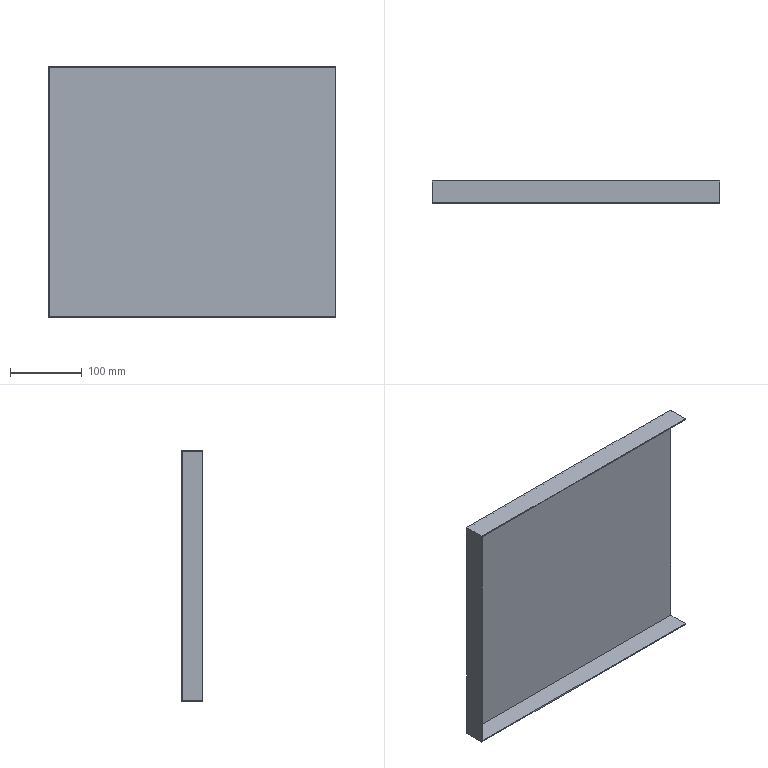Part | STEP file | B-BAN1_1-2 | 1 solid | 10 faces | box 400 x 30 x 350 mm | volume 259034 mm3 | plane 10
STEP:
#1=CARTESIAN_POINT('',(200.,30.,-175.));
#2=VERTEX_POINT('',#1);
#3=CARTESIAN_POINT('',(-200.,30.,-175.));
#4=VERTEX_POINT('',#3);
#5=CARTESIAN_POINT('',(0.,30.,-175.));
#6=DIRECTION('',(-1.,0.,0.));
#7=VECTOR('',#6,1000.);
#8=LINE('',#5,#7);
#9=EDGE_CURVE('',#2,#4,#8,.T.);
#10=ORIENTED_EDGE('',*,*,#9,.T.);
#11=CARTESIAN_POINT('',(-200.,30.,175.));
#12=VERTEX_POINT('',#11);
#13=CARTESIAN_POINT('',(-200.,30.,0.));
#14=DIRECTION('',(0.,0.,1.));
#15=VECTOR('',#14,1000.);
#16=LINE('',#13,#15);
#17=EDGE_CURVE('',#4,#12,#16,.T.);
#18=ORIENTED_EDGE('',*,*,#17,.T.);
#19=CARTESIAN_POINT('',(200.,30.,175.));
#20=VERTEX_POINT('',#19);
#21=CARTESIAN_POINT('',(0.,30.,175.));
#22=DIRECTION('',(1.,0.,0.));
#23=VECTOR('',#22,1000.);
#24=LINE('',#21,#23);
#25=EDGE_CURVE('',#12,#20,#24,.T.);
#26=ORIENTED_EDGE('',*,*,#25,.T.);
#27=CARTESIAN_POINT('',(200.,30.,0.));
#28=DIRECTION('',(0.,0.,-1.));
#29=VECTOR('',#28,1000.);
#30=LINE('',#27,#29);
#31=EDGE_CURVE('',#20,#2,#30,.T.);
#32=ORIENTED_EDGE('',*,*,#31,.T.);
#33=EDGE_LOOP('',(#10,#18,#26,#32));
#34=FACE_OUTER_BOUND('',#33,.T.);
#35=CARTESIAN_POINT('',(0.,30.,0.));
#36=DIRECTION('',(0.,1.,0.));
#37=DIRECTION('',(0.,0.,1.));
#38=AXIS2_PLACEMENT_3D('',#35,#36,#37);
#39=PLANE('',#38);
#40=ADVANCED_FACE('',(#34),#39,.T.);
#41=CARTESIAN_POINT('',(-200.,0.,-175.));
#42=VERTEX_POINT('',#41);
#43=CARTESIAN_POINT('',(-200.,0.,-175.));
#44=DIRECTION('',(0.,-1.,0.));
#45=VECTOR('',#44,1000.);
#46=LINE('',#43,#45);
#47=EDGE_CURVE('',#4,#42,#46,.T.);
#48=ORIENTED_EDGE('',*,*,#47,.T.);
#49=CARTESIAN_POINT('',(-200.,0.,175.));
#50=VERTEX_POINT('',#49);
#51=CARTESIAN_POINT('',(-200.,0.,-175.));
#52=DIRECTION('',(0.,0.,1.));
#53=VECTOR('',#52,1000.);
#54=LINE('',#51,#53);
#55=EDGE_CURVE('',#42,#50,#54,.T.);
#56=ORIENTED_EDGE('',*,*,#55,.T.);
#57=CARTESIAN_POINT('',(-200.,0.,175.));
#58=DIRECTION('',(0.,1.,0.));
#59=VECTOR('',#58,1000.);
#60=LINE('',#57,#59);
#61=EDGE_CURVE('',#50,#12,#60,.T.);
#62=ORIENTED_EDGE('',*,*,#61,.T.);
#63=ORIENTED_EDGE('',*,*,#17,.F.);
#64=EDGE_LOOP('',(#48,#56,#62,#63));
#65=FACE_OUTER_BOUND('',#64,.T.);
#66=CARTESIAN_POINT('',(-200.,0.,-175.));
#67=DIRECTION('',(-1.,0.,0.));
#68=DIRECTION('',(0.,0.,1.));
#69=AXIS2_PLACEMENT_3D('',#66,#67,#68);
#70=PLANE('',#69);
#71=ADVANCED_FACE('',(#65),#70,.T.);
#72=CARTESIAN_POINT('',(200.,0.,-175.));
#73=VERTEX_POINT('',#72);
#74=CARTESIAN_POINT('',(200.,0.,-175.));
#75=DIRECTION('',(0.,-1.,0.));
#76=VECTOR('',#75,1000.);
#77=LINE('',#74,#76);
#78=EDGE_CURVE('',#2,#73,#77,.T.);
#79=ORIENTED_EDGE('',*,*,#78,.T.);
#80=CARTESIAN_POINT('',(200.,0.,-175.));
#81=DIRECTION('',(-1.,0.,0.));
#82=VECTOR('',#81,1000.);
#83=LINE('',#80,#82);
#84=EDGE_CURVE('',#73,#42,#83,.T.);
#85=ORIENTED_EDGE('',*,*,#84,.T.);
#86=ORIENTED_EDGE('',*,*,#47,.F.);
#87=ORIENTED_EDGE('',*,*,#9,.F.);
#88=EDGE_LOOP('',(#79,#85,#86,#87));
#89=FACE_OUTER_BOUND('',#88,.T.);
#90=CARTESIAN_POINT('',(200.,0.,-175.));
#91=DIRECTION('',(0.,0.,-1.));
#92=DIRECTION('',(-1.,0.,0.));
#93=AXIS2_PLACEMENT_3D('',#90,#91,#92);
#94=PLANE('',#93);
#95=ADVANCED_FACE('',(#89),#94,.T.);
#96=CARTESIAN_POINT('',(200.,0.,173.5));
#97=VERTEX_POINT('',#96);
#98=CARTESIAN_POINT('',(200.,28.5,173.5));
#99=VERTEX_POINT('',#98);
#100=CARTESIAN_POINT('',(200.,0.,173.5));
#101=DIRECTION('',(0.,1.,0.));
#102=VECTOR('',#101,1000.);
#103=LINE('',#100,#102);
#104=EDGE_CURVE('',#97,#99,#103,.T.);
#105=ORIENTED_EDGE('',*,*,#104,.T.);
#106=CARTESIAN_POINT('',(200.,28.5,-173.5));
#107=VERTEX_POINT('',#106);
#108=CARTESIAN_POINT('',(200.,28.5,175.));
#109=DIRECTION('',(0.,0.,-1.));
#110=VECTOR('',#109,1000.);
#111=LINE('',#108,#110);
#112=EDGE_CURVE('',#99,#107,#111,.T.);
#113=ORIENTED_EDGE('',*,*,#112,.T.);
#114=CARTESIAN_POINT('',(200.,0.,-173.5));
#115=VERTEX_POINT('',#114);
#116=CARTESIAN_POINT('',(200.,0.,-173.5));
#117=DIRECTION('',(0.,-1.,0.));
#118=VECTOR('',#117,1000.);
#119=LINE('',#116,#118);
#120=EDGE_CURVE('',#107,#115,#119,.T.);
#121=ORIENTED_EDGE('',*,*,#120,.T.);
#122=CARTESIAN_POINT('',(200.,0.,175.));
#123=DIRECTION('',(0.,0.,-1.));
#124=VECTOR('',#123,1000.);
#125=LINE('',#122,#124);
#126=EDGE_CURVE('',#115,#73,#125,.T.);
#127=ORIENTED_EDGE('',*,*,#126,.T.);
#128=ORIENTED_EDGE('',*,*,#78,.F.);
#129=ORIENTED_EDGE('',*,*,#31,.F.);
#130=CARTESIAN_POINT('',(200.,0.,175.));
#131=VERTEX_POINT('',#130);
#132=CARTESIAN_POINT('',(200.,0.,175.));
#133=DIRECTION('',(0.,-1.,0.));
#134=VECTOR('',#133,1000.);
#135=LINE('',#132,#134);
#136=EDGE_CURVE('',#20,#131,#135,.T.);
#137=ORIENTED_EDGE('',*,*,#136,.T.);
#138=CARTESIAN_POINT('',(200.,0.,175.));
#139=DIRECTION('',(0.,0.,-1.));
#140=VECTOR('',#139,1000.);
#141=LINE('',#138,#140);
#142=EDGE_CURVE('',#131,#97,#141,.T.);
#143=ORIENTED_EDGE('',*,*,#142,.T.);
#144=EDGE_LOOP('',(#105,#113,#121,#127,#128,#129,#137,#143));
#145=FACE_OUTER_BOUND('',#144,.T.);
#146=CARTESIAN_POINT('',(200.,0.,175.));
#147=DIRECTION('',(1.,0.,0.));
#148=DIRECTION('',(0.,0.,-1.));
#149=AXIS2_PLACEMENT_3D('',#146,#147,#148);
#150=PLANE('',#149);
#151=ADVANCED_FACE('',(#145),#150,.T.);
#152=ORIENTED_EDGE('',*,*,#61,.F.);
#153=CARTESIAN_POINT('',(-200.,0.,175.));
#154=DIRECTION('',(1.,0.,0.));
#155=VECTOR('',#154,1000.);
#156=LINE('',#153,#155);
#157=EDGE_CURVE('',#50,#131,#156,.T.);
#158=ORIENTED_EDGE('',*,*,#157,.T.);
#159=ORIENTED_EDGE('',*,*,#136,.F.);
#160=ORIENTED_EDGE('',*,*,#25,.F.);
#161=EDGE_LOOP('',(#152,#158,#159,#160));
#162=FACE_OUTER_BOUND('',#161,.T.);
#163=CARTESIAN_POINT('',(-200.,0.,175.));
#164=DIRECTION('',(0.,0.,1.));
#165=DIRECTION('',(1.,0.,0.));
#166=AXIS2_PLACEMENT_3D('',#163,#164,#165);
#167=PLANE('',#166);
#168=ADVANCED_FACE('',(#162),#167,.T.);
#169=ORIENTED_EDGE('',*,*,#142,.F.);
#170=ORIENTED_EDGE('',*,*,#157,.F.);
#171=ORIENTED_EDGE('',*,*,#55,.F.);
#172=ORIENTED_EDGE('',*,*,#84,.F.);
#173=ORIENTED_EDGE('',*,*,#126,.F.);
#174=CARTESIAN_POINT('',(-198.5,0.,-173.5));
#175=VERTEX_POINT('',#174);
#176=CARTESIAN_POINT('',(0.,0.,-173.5));
#177=DIRECTION('',(1.,0.,0.));
#178=VECTOR('',#177,1000.);
#179=LINE('',#176,#178);
#180=EDGE_CURVE('',#175,#115,#179,.T.);
#181=ORIENTED_EDGE('',*,*,#180,.F.);
#182=CARTESIAN_POINT('',(-198.5,0.,173.5));
#183=VERTEX_POINT('',#182);
#184=CARTESIAN_POINT('',(-198.5,0.,0.));
#185=DIRECTION('',(0.,0.,-1.));
#186=VECTOR('',#185,1000.);
#187=LINE('',#184,#186);
#188=EDGE_CURVE('',#183,#175,#187,.T.);
#189=ORIENTED_EDGE('',*,*,#188,.F.);
#190=CARTESIAN_POINT('',(0.,0.,173.5));
#191=DIRECTION('',(-1.,0.,0.));
#192=VECTOR('',#191,1000.);
#193=LINE('',#190,#192);
#194=EDGE_CURVE('',#97,#183,#193,.T.);
#195=ORIENTED_EDGE('',*,*,#194,.F.);
#196=EDGE_LOOP('',(#169,#170,#171,#172,#173,#181,#189,#195));
#197=FACE_OUTER_BOUND('',#196,.T.);
#198=CARTESIAN_POINT('',(0.,0.,0.));
#199=DIRECTION('',(0.,1.,0.));
#200=DIRECTION('',(0.,0.,1.));
#201=AXIS2_PLACEMENT_3D('',#198,#199,#200);
#202=PLANE('',#201);
#203=ADVANCED_FACE('',(#197),#202,.F.);
#204=CARTESIAN_POINT('',(-198.5,28.5,-173.5));
#205=VERTEX_POINT('',#204);
#206=CARTESIAN_POINT('',(-198.5,28.5,173.5));
#207=VERTEX_POINT('',#206);
#208=CARTESIAN_POINT('',(-198.5,28.5,0.));
#209=DIRECTION('',(0.,0.,1.));
#210=VECTOR('',#209,1000.);
#211=LINE('',#208,#210);
#212=EDGE_CURVE('',#205,#207,#211,.T.);
#213=ORIENTED_EDGE('',*,*,#212,.F.);
#214=CARTESIAN_POINT('',(0.,28.5,-173.5));
#215=DIRECTION('',(-1.,0.,0.));
#216=VECTOR('',#215,1000.);
#217=LINE('',#214,#216);
#218=EDGE_CURVE('',#107,#205,#217,.T.);
#219=ORIENTED_EDGE('',*,*,#218,.F.);
#220=ORIENTED_EDGE('',*,*,#112,.F.);
#221=CARTESIAN_POINT('',(0.,28.5,173.5));
#222=DIRECTION('',(1.,0.,0.));
#223=VECTOR('',#222,1000.);
#224=LINE('',#221,#223);
#225=EDGE_CURVE('',#207,#99,#224,.T.);
#226=ORIENTED_EDGE('',*,*,#225,.F.);
#227=EDGE_LOOP('',(#213,#219,#220,#226));
#228=FACE_OUTER_BOUND('',#227,.T.);
#229=CARTESIAN_POINT('',(0.,28.5,0.));
#230=DIRECTION('',(0.,1.,0.));
#231=DIRECTION('',(0.,0.,1.));
#232=AXIS2_PLACEMENT_3D('',#229,#230,#231);
#233=PLANE('',#232);
#234=ADVANCED_FACE('',(#228),#233,.F.);
#235=ORIENTED_EDGE('',*,*,#225,.T.);
#236=ORIENTED_EDGE('',*,*,#104,.F.);
#237=ORIENTED_EDGE('',*,*,#194,.T.);
#238=CARTESIAN_POINT('',(-198.5,0.,173.5));
#239=DIRECTION('',(0.,-1.,0.));
#240=VECTOR('',#239,1000.);
#241=LINE('',#238,#240);
#242=EDGE_CURVE('',#207,#183,#241,.T.);
#243=ORIENTED_EDGE('',*,*,#242,.F.);
#244=EDGE_LOOP('',(#235,#236,#237,#243));
#245=FACE_OUTER_BOUND('',#244,.T.);
#246=CARTESIAN_POINT('',(-200.,0.,173.5));
#247=DIRECTION('',(0.,0.,1.));
#248=DIRECTION('',(1.,0.,0.));
#249=AXIS2_PLACEMENT_3D('',#246,#247,#248);
#250=PLANE('',#249);
#251=ADVANCED_FACE('',(#245),#250,.F.);
#252=ORIENTED_EDGE('',*,*,#218,.T.);
#253=CARTESIAN_POINT('',(-198.5,0.,-173.5));
#254=DIRECTION('',(0.,1.,0.));
#255=VECTOR('',#254,1000.);
#256=LINE('',#253,#255);
#257=EDGE_CURVE('',#175,#205,#256,.T.);
#258=ORIENTED_EDGE('',*,*,#257,.F.);
#259=ORIENTED_EDGE('',*,*,#180,.T.);
#260=ORIENTED_EDGE('',*,*,#120,.F.);
#261=EDGE_LOOP('',(#252,#258,#259,#260));
#262=FACE_OUTER_BOUND('',#261,.T.);
#263=CARTESIAN_POINT('',(200.,0.,-173.5));
#264=DIRECTION('',(0.,0.,-1.));
#265=DIRECTION('',(-1.,0.,0.));
#266=AXIS2_PLACEMENT_3D('',#263,#264,#265);
#267=PLANE('',#266);
#268=ADVANCED_FACE('',(#262),#267,.F.);
#269=ORIENTED_EDGE('',*,*,#212,.T.);
#270=ORIENTED_EDGE('',*,*,#242,.T.);
#271=ORIENTED_EDGE('',*,*,#188,.T.);
#272=ORIENTED_EDGE('',*,*,#257,.T.);
#273=EDGE_LOOP('',(#269,#270,#271,#272));
#274=FACE_OUTER_BOUND('',#273,.T.);
#275=CARTESIAN_POINT('',(-198.5,0.,-175.));
#276=DIRECTION('',(-1.,0.,0.));
#277=DIRECTION('',(0.,0.,1.));
#278=AXIS2_PLACEMENT_3D('',#275,#276,#277);
#279=PLANE('',#278);
#280=ADVANCED_FACE('',(#274),#279,.F.);
#281=CLOSED_SHELL('',(#40,#71,#95,#151,#168,#203,#234,#251,#268,#280));
#282=MANIFOLD_SOLID_BREP('',#281);
#283=CARTESIAN_POINT('',(0.,0.,0.));
#284=DIRECTION('',(0.,0.,1.));
#285=DIRECTION('',(1.,0.,0.));
#286=AXIS2_PLACEMENT_3D('',#283,#284,#285);
#287=(LENGTH_UNIT()NAMED_UNIT(*)SI_UNIT(.MILLI.,.METRE.));
#288=UNCERTAINTY_MEASURE_WITH_UNIT(LENGTH_MEASURE(0.00001),#287,'','');
#289=(NAMED_UNIT(*)PLANE_ANGLE_UNIT()SI_UNIT($,.RADIAN.));
#290=(NAMED_UNIT(*)SI_UNIT($,.STERADIAN.)SOLID_ANGLE_UNIT());
#291=(GEOMETRIC_REPRESENTATION_CONTEXT(3)GLOBAL_UNCERTAINTY_ASSIGNED_CONTEXT((#288))GLOBAL_UNIT_ASSIGNED_CONTEXT((#287,#289,#290))REPRESENTATION_CONTEXT('',''));
#292=ADVANCED_BREP_SHAPE_REPRESENTATION('',(#282,#286),#291);